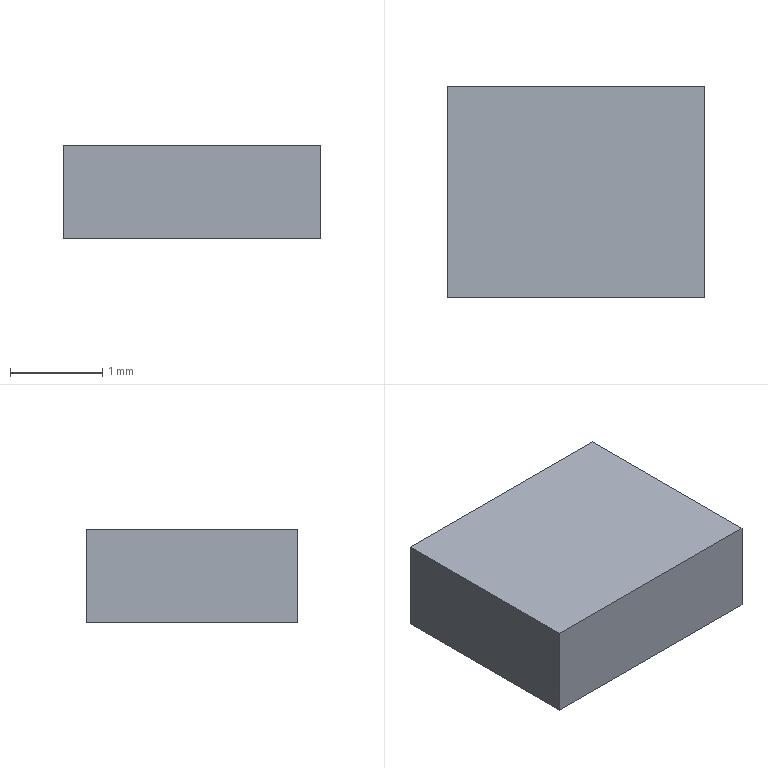Part | Creo | 1 solid | 6 faces | box 2.8 x 2.3 x 1.02 mm | volume 6.569 mm3 | plane 6
STEP:
#1=CARTESIAN_POINT('',(0.,0.,0.));
#2=DIRECTION('',(0.,0.,1.));
#3=DIRECTION('',(1.,0.,0.));
#4=AXIS2_PLACEMENT_3D('',#1,#2,#3);
#5=CARTESIAN_POINT('',(-1.4,1.15,0.));
#6=VERTEX_POINT('',#5);
#7=CARTESIAN_POINT('',(-1.4,-1.15,0.));
#8=VERTEX_POINT('',#7);
#9=CARTESIAN_POINT('',(-1.4,1.15,0.));
#10=DIRECTION('',(0.,-1.,0.));
#11=VECTOR('',#10,2.3);
#12=LINE('',#9,#11);
#13=EDGE_CURVE('',#6,#8,#12,.T.);
#14=ORIENTED_EDGE('',*,*,#13,.T.);
#15=CARTESIAN_POINT('',(1.4,-1.15,0.));
#16=VERTEX_POINT('',#15);
#17=CARTESIAN_POINT('',(-1.4,-1.15,0.));
#18=DIRECTION('',(1.,0.,0.));
#19=VECTOR('',#18,2.8);
#20=LINE('',#17,#19);
#21=EDGE_CURVE('',#8,#16,#20,.T.);
#22=ORIENTED_EDGE('',*,*,#21,.T.);
#23=CARTESIAN_POINT('',(1.4,1.15,0.));
#24=VERTEX_POINT('',#23);
#25=CARTESIAN_POINT('',(1.4,-1.15,0.));
#26=DIRECTION('',(0.,1.,0.));
#27=VECTOR('',#26,2.3);
#28=LINE('',#25,#27);
#29=EDGE_CURVE('',#16,#24,#28,.T.);
#30=ORIENTED_EDGE('',*,*,#29,.T.);
#31=CARTESIAN_POINT('',(1.4,1.15,0.));
#32=DIRECTION('',(-1.,0.,0.));
#33=VECTOR('',#32,2.8);
#34=LINE('',#31,#33);
#35=EDGE_CURVE('',#24,#6,#34,.T.);
#36=ORIENTED_EDGE('',*,*,#35,.T.);
#37=EDGE_LOOP('',(#14,#22,#30,#36));
#38=FACE_OUTER_BOUND('',#37,.F.);
#39=CARTESIAN_POINT('',(0.,0.,0.));
#40=DIRECTION('',(0.,0.,1.));
#41=DIRECTION('',(1.,0.,0.));
#42=AXIS2_PLACEMENT_3D('',#39,#40,#41);
#43=PLANE('',#42);
#44=ADVANCED_FACE('',(#38),#43,.F.);
#45=ORIENTED_EDGE('',*,*,#13,.F.);
#46=CARTESIAN_POINT('',(-1.4,1.15,1.02));
#47=VERTEX_POINT('',#46);
#48=CARTESIAN_POINT('',(-1.4,1.15,0.));
#49=DIRECTION('',(0.,0.,1.));
#50=VECTOR('',#49,1.02);
#51=LINE('',#48,#50);
#52=EDGE_CURVE('',#6,#47,#51,.T.);
#53=ORIENTED_EDGE('',*,*,#52,.T.);
#54=CARTESIAN_POINT('',(-1.4,-1.15,1.02));
#55=VERTEX_POINT('',#54);
#56=CARTESIAN_POINT('',(-1.4,1.15,1.02));
#57=DIRECTION('',(0.,-1.,0.));
#58=VECTOR('',#57,2.3);
#59=LINE('',#56,#58);
#60=EDGE_CURVE('',#47,#55,#59,.T.);
#61=ORIENTED_EDGE('',*,*,#60,.T.);
#62=CARTESIAN_POINT('',(-1.4,-1.15,0.));
#63=DIRECTION('',(0.,0.,1.));
#64=VECTOR('',#63,1.02);
#65=LINE('',#62,#64);
#66=EDGE_CURVE('',#8,#55,#65,.T.);
#67=ORIENTED_EDGE('',*,*,#66,.F.);
#68=EDGE_LOOP('',(#45,#53,#61,#67));
#69=FACE_OUTER_BOUND('',#68,.F.);
#70=CARTESIAN_POINT('',(-1.4,1.15,0.));
#71=DIRECTION('',(-1.,0.,0.));
#72=DIRECTION('',(0.,-1.,0.));
#73=AXIS2_PLACEMENT_3D('',#70,#71,#72);
#74=PLANE('',#73);
#75=ADVANCED_FACE('',(#69),#74,.T.);
#76=ORIENTED_EDGE('',*,*,#35,.F.);
#77=CARTESIAN_POINT('',(1.4,1.15,1.02));
#78=VERTEX_POINT('',#77);
#79=CARTESIAN_POINT('',(1.4,1.15,0.));
#80=DIRECTION('',(0.,0.,1.));
#81=VECTOR('',#80,1.02);
#82=LINE('',#79,#81);
#83=EDGE_CURVE('',#24,#78,#82,.T.);
#84=ORIENTED_EDGE('',*,*,#83,.T.);
#85=CARTESIAN_POINT('',(1.4,1.15,1.02));
#86=DIRECTION('',(-1.,0.,0.));
#87=VECTOR('',#86,2.8);
#88=LINE('',#85,#87);
#89=EDGE_CURVE('',#78,#47,#88,.T.);
#90=ORIENTED_EDGE('',*,*,#89,.T.);
#91=ORIENTED_EDGE('',*,*,#52,.F.);
#92=EDGE_LOOP('',(#76,#84,#90,#91));
#93=FACE_OUTER_BOUND('',#92,.F.);
#94=CARTESIAN_POINT('',(1.4,1.15,0.));
#95=DIRECTION('',(0.,1.,0.));
#96=DIRECTION('',(-1.,0.,0.));
#97=AXIS2_PLACEMENT_3D('',#94,#95,#96);
#98=PLANE('',#97);
#99=ADVANCED_FACE('',(#93),#98,.T.);
#100=ORIENTED_EDGE('',*,*,#29,.F.);
#101=CARTESIAN_POINT('',(1.4,-1.15,1.02));
#102=VERTEX_POINT('',#101);
#103=CARTESIAN_POINT('',(1.4,-1.15,0.));
#104=DIRECTION('',(0.,0.,1.));
#105=VECTOR('',#104,1.02);
#106=LINE('',#103,#105);
#107=EDGE_CURVE('',#16,#102,#106,.T.);
#108=ORIENTED_EDGE('',*,*,#107,.T.);
#109=CARTESIAN_POINT('',(1.4,-1.15,1.02));
#110=DIRECTION('',(0.,1.,0.));
#111=VECTOR('',#110,2.3);
#112=LINE('',#109,#111);
#113=EDGE_CURVE('',#102,#78,#112,.T.);
#114=ORIENTED_EDGE('',*,*,#113,.T.);
#115=ORIENTED_EDGE('',*,*,#83,.F.);
#116=EDGE_LOOP('',(#100,#108,#114,#115));
#117=FACE_OUTER_BOUND('',#116,.F.);
#118=CARTESIAN_POINT('',(1.4,-1.15,0.));
#119=DIRECTION('',(1.,0.,0.));
#120=DIRECTION('',(0.,1.,0.));
#121=AXIS2_PLACEMENT_3D('',#118,#119,#120);
#122=PLANE('',#121);
#123=ADVANCED_FACE('',(#117),#122,.T.);
#124=ORIENTED_EDGE('',*,*,#21,.F.);
#125=ORIENTED_EDGE('',*,*,#66,.T.);
#126=CARTESIAN_POINT('',(-1.4,-1.15,1.02));
#127=DIRECTION('',(1.,0.,0.));
#128=VECTOR('',#127,2.8);
#129=LINE('',#126,#128);
#130=EDGE_CURVE('',#55,#102,#129,.T.);
#131=ORIENTED_EDGE('',*,*,#130,.T.);
#132=ORIENTED_EDGE('',*,*,#107,.F.);
#133=EDGE_LOOP('',(#124,#125,#131,#132));
#134=FACE_OUTER_BOUND('',#133,.F.);
#135=CARTESIAN_POINT('',(-1.4,-1.15,0.));
#136=DIRECTION('',(0.,-1.,0.));
#137=DIRECTION('',(1.,0.,0.));
#138=AXIS2_PLACEMENT_3D('',#135,#136,#137);
#139=PLANE('',#138);
#140=ADVANCED_FACE('',(#134),#139,.T.);
#141=ORIENTED_EDGE('',*,*,#60,.F.);
#142=ORIENTED_EDGE('',*,*,#89,.F.);
#143=ORIENTED_EDGE('',*,*,#113,.F.);
#144=ORIENTED_EDGE('',*,*,#130,.F.);
#145=EDGE_LOOP('',(#141,#142,#143,#144));
#146=FACE_OUTER_BOUND('',#145,.F.);
#147=CARTESIAN_POINT('',(0.,0.,1.02));
#148=DIRECTION('',(0.,0.,1.));
#149=DIRECTION('',(1.,0.,0.));
#150=AXIS2_PLACEMENT_3D('',#147,#148,#149);
#151=PLANE('',#150);
#152=ADVANCED_FACE('',(#146),#151,.T.);
#153=CLOSED_SHELL('',(#44,#75,#99,#123,#140,#152));
#154=MANIFOLD_SOLID_BREP('',#153);
#155=(LENGTH_UNIT()NAMED_UNIT(*)SI_UNIT(.MILLI.,.METRE.));
#156=UNCERTAINTY_MEASURE_WITH_UNIT(LENGTH_MEASURE(0.0003764),#155,'','');
#157=(NAMED_UNIT(*)PLANE_ANGLE_UNIT()SI_UNIT($,.RADIAN.));
#158=PLANE_ANGLE_MEASURE_WITH_UNIT(PLANE_ANGLE_MEASURE(0.01745),#157);
#159=(CONVERSION_BASED_UNIT('DEGREE',#158)NAMED_UNIT(*)PLANE_ANGLE_UNIT());
#160=(NAMED_UNIT(*)SI_UNIT($,.STERADIAN.)SOLID_ANGLE_UNIT());
#161=(GEOMETRIC_REPRESENTATION_CONTEXT(3)GLOBAL_UNCERTAINTY_ASSIGNED_CONTEXT((#156))GLOBAL_UNIT_ASSIGNED_CONTEXT((#155,#159,#160))REPRESENTATION_CONTEXT('',''));
#162=ADVANCED_BREP_SHAPE_REPRESENTATION('',(#4,#154),#161);